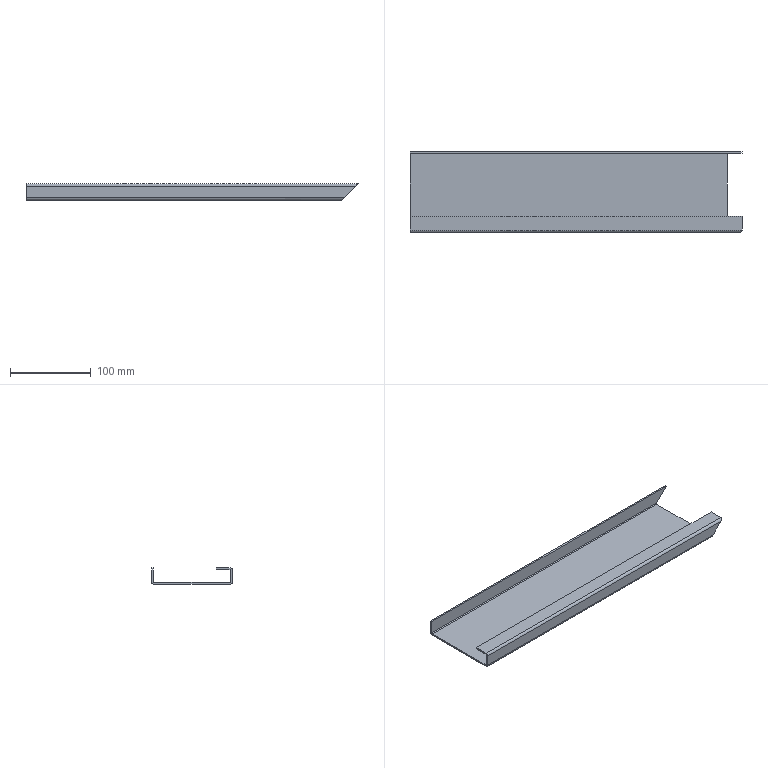Part | STEP file | 护栏90度踢脚Plate-2 | 1 solid | 18 faces | box 410 x 100 x 20 mm | volume 119752 mm3 | plane 12 | cylinder 6 | commonest cylinder face diameters 2 x3 6 x3